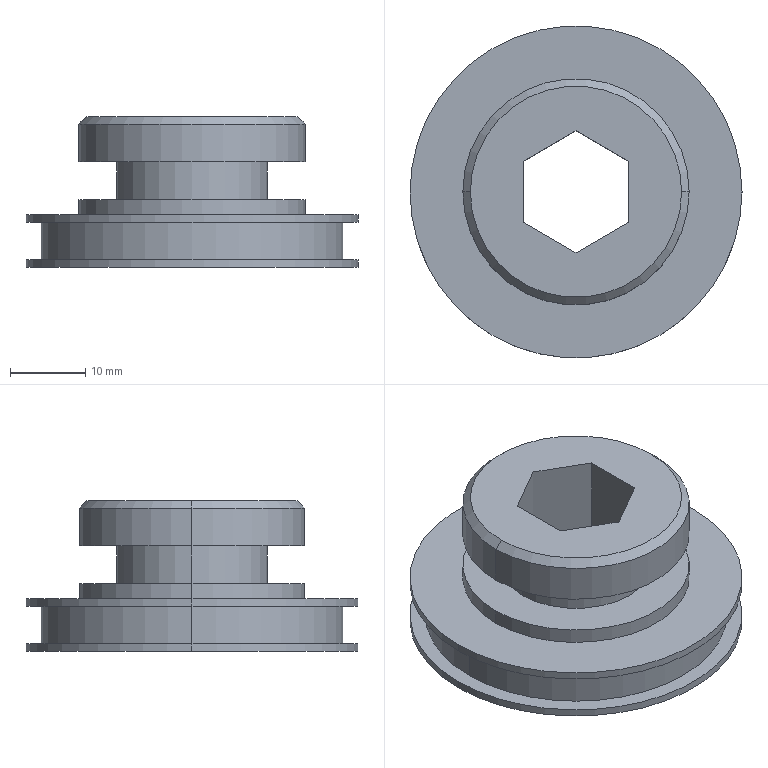Part | STEP file | 103-01-0007 | 1 solid | 27 faces | box 44 x 44 x 20 mm | volume 13109 mm3 | plane 13 | cylinder 12 | cone 2 | commonest cylinder face diameters 30 x4 44 x4 20 x2 40 x2